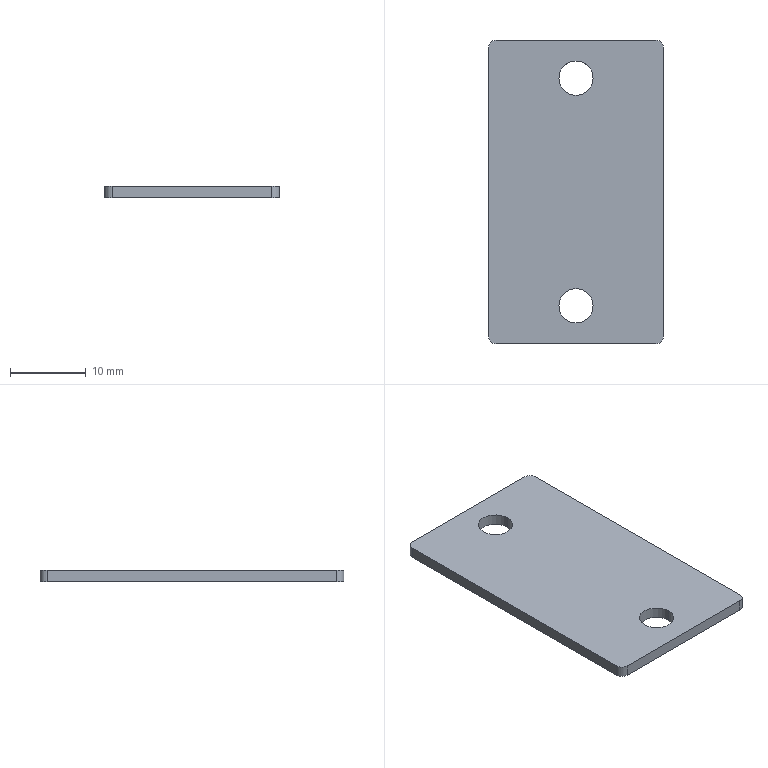Part | STEP file | LE-MX-A-P2_PN_0009 | 1 solid | 14 faces | box 23 x 40 x 1.5 mm | volume 1331 mm3 | cylinder 8 | plane 6 | commonest cylinder face diameters 2 x4 4.5 x4
STEP:
#1=CARTESIAN_POINT('',(2.25,15.,1.5));
#2=VERTEX_POINT('',#1);
#3=CARTESIAN_POINT('',(-2.25,15.,1.5));
#4=VERTEX_POINT('',#3);
#5=CARTESIAN_POINT('',(0.,15.,1.5));
#6=DIRECTION('',(0.,0.,-1.));
#7=DIRECTION('',(-1.,0.,0.));
#8=AXIS2_PLACEMENT_3D('',#5,#6,#7);
#9=CIRCLE('',#8,2.25);
#10=EDGE_CURVE('',#2,#4,#9,.T.);
#11=ORIENTED_EDGE('',*,*,#10,.F.);
#12=CARTESIAN_POINT('',(2.25,15.,0.));
#13=VERTEX_POINT('',#12);
#14=CARTESIAN_POINT('',(2.25,15.,1.5));
#15=DIRECTION('',(0.,0.,-1.));
#16=VECTOR('',#15,1000.);
#17=LINE('',#14,#16);
#18=EDGE_CURVE('',#2,#13,#17,.T.);
#19=ORIENTED_EDGE('',*,*,#18,.T.);
#20=CARTESIAN_POINT('',(-2.25,15.,0.));
#21=VERTEX_POINT('',#20);
#22=CARTESIAN_POINT('',(0.,15.,0.));
#23=DIRECTION('',(0.,0.,1.));
#24=DIRECTION('',(-1.,0.,0.));
#25=AXIS2_PLACEMENT_3D('',#22,#23,#24);
#26=CIRCLE('',#25,2.25);
#27=EDGE_CURVE('',#21,#13,#26,.T.);
#28=ORIENTED_EDGE('',*,*,#27,.F.);
#29=CARTESIAN_POINT('',(-2.25,15.,1.5));
#30=DIRECTION('',(0.,0.,-1.));
#31=VECTOR('',#30,1000.);
#32=LINE('',#29,#31);
#33=EDGE_CURVE('',#4,#21,#32,.T.);
#34=ORIENTED_EDGE('',*,*,#33,.F.);
#35=EDGE_LOOP('',(#11,#19,#28,#34));
#36=FACE_OUTER_BOUND('',#35,.T.);
#37=CARTESIAN_POINT('',(0.,15.,1.5));
#38=DIRECTION('',(0.,0.,-1.));
#39=DIRECTION('',(-1.,0.,0.));
#40=AXIS2_PLACEMENT_3D('',#37,#38,#39);
#41=CYLINDRICAL_SURFACE('',#40,2.25);
#42=ADVANCED_FACE('',(#36),#41,.F.);
#43=CARTESIAN_POINT('',(2.25,-15.,1.5));
#44=VERTEX_POINT('',#43);
#45=CARTESIAN_POINT('',(-2.25,-15.,1.5));
#46=VERTEX_POINT('',#45);
#47=CARTESIAN_POINT('',(0.,-15.,1.5));
#48=DIRECTION('',(0.,0.,-1.));
#49=DIRECTION('',(-1.,0.,0.));
#50=AXIS2_PLACEMENT_3D('',#47,#48,#49);
#51=CIRCLE('',#50,2.25);
#52=EDGE_CURVE('',#44,#46,#51,.T.);
#53=ORIENTED_EDGE('',*,*,#52,.F.);
#54=CARTESIAN_POINT('',(2.25,-15.,0.));
#55=VERTEX_POINT('',#54);
#56=CARTESIAN_POINT('',(2.25,-15.,1.5));
#57=DIRECTION('',(0.,0.,-1.));
#58=VECTOR('',#57,1000.);
#59=LINE('',#56,#58);
#60=EDGE_CURVE('',#44,#55,#59,.T.);
#61=ORIENTED_EDGE('',*,*,#60,.T.);
#62=CARTESIAN_POINT('',(-2.25,-15.,0.));
#63=VERTEX_POINT('',#62);
#64=CARTESIAN_POINT('',(0.,-15.,0.));
#65=DIRECTION('',(0.,0.,1.));
#66=DIRECTION('',(-1.,0.,0.));
#67=AXIS2_PLACEMENT_3D('',#64,#65,#66);
#68=CIRCLE('',#67,2.25);
#69=EDGE_CURVE('',#63,#55,#68,.T.);
#70=ORIENTED_EDGE('',*,*,#69,.F.);
#71=CARTESIAN_POINT('',(-2.25,-15.,1.5));
#72=DIRECTION('',(0.,0.,-1.));
#73=VECTOR('',#72,1000.);
#74=LINE('',#71,#73);
#75=EDGE_CURVE('',#46,#63,#74,.T.);
#76=ORIENTED_EDGE('',*,*,#75,.F.);
#77=EDGE_LOOP('',(#53,#61,#70,#76));
#78=FACE_OUTER_BOUND('',#77,.T.);
#79=CARTESIAN_POINT('',(0.,-15.,1.5));
#80=DIRECTION('',(0.,0.,-1.));
#81=DIRECTION('',(-1.,0.,0.));
#82=AXIS2_PLACEMENT_3D('',#79,#80,#81);
#83=CYLINDRICAL_SURFACE('',#82,2.25);
#84=ADVANCED_FACE('',(#78),#83,.F.);
#85=CARTESIAN_POINT('',(0.,15.,1.5));
#86=DIRECTION('',(0.,0.,-1.));
#87=DIRECTION('',(-1.,0.,0.));
#88=AXIS2_PLACEMENT_3D('',#85,#86,#87);
#89=CIRCLE('',#88,2.25);
#90=EDGE_CURVE('',#4,#2,#89,.T.);
#91=ORIENTED_EDGE('',*,*,#90,.T.);
#92=ORIENTED_EDGE('',*,*,#10,.T.);
#93=EDGE_LOOP('',(#91,#92));
#94=FACE_BOUND('',#93,.T.);
#95=CARTESIAN_POINT('',(-10.5,20.,1.5));
#96=VERTEX_POINT('',#95);
#97=CARTESIAN_POINT('',(-11.5,19.,1.5));
#98=VERTEX_POINT('',#97);
#99=CARTESIAN_POINT('',(-10.5,19.,1.5));
#100=DIRECTION('',(0.,0.,1.));
#101=DIRECTION('',(-1.,0.,0.));
#102=AXIS2_PLACEMENT_3D('',#99,#100,#101);
#103=CIRCLE('',#102,1.);
#104=EDGE_CURVE('',#96,#98,#103,.T.);
#105=ORIENTED_EDGE('',*,*,#104,.T.);
#106=CARTESIAN_POINT('',(-11.5,-19.,1.5));
#107=VERTEX_POINT('',#106);
#108=CARTESIAN_POINT('',(-11.5,-19.,1.5));
#109=DIRECTION('',(0.,-1.,0.));
#110=VECTOR('',#109,1000.);
#111=LINE('',#108,#110);
#112=EDGE_CURVE('',#98,#107,#111,.T.);
#113=ORIENTED_EDGE('',*,*,#112,.T.);
#114=CARTESIAN_POINT('',(-10.5,-20.,1.5));
#115=VERTEX_POINT('',#114);
#116=CARTESIAN_POINT('',(-10.5,-19.,1.5));
#117=DIRECTION('',(0.,0.,1.));
#118=DIRECTION('',(-1.,0.,0.));
#119=AXIS2_PLACEMENT_3D('',#116,#117,#118);
#120=CIRCLE('',#119,1.);
#121=EDGE_CURVE('',#107,#115,#120,.T.);
#122=ORIENTED_EDGE('',*,*,#121,.T.);
#123=CARTESIAN_POINT('',(10.5,-20.,1.5));
#124=VERTEX_POINT('',#123);
#125=CARTESIAN_POINT('',(-10.5,-20.,1.5));
#126=DIRECTION('',(1.,0.,0.));
#127=VECTOR('',#126,1000.);
#128=LINE('',#125,#127);
#129=EDGE_CURVE('',#115,#124,#128,.T.);
#130=ORIENTED_EDGE('',*,*,#129,.T.);
#131=CARTESIAN_POINT('',(11.5,-19.,1.5));
#132=VERTEX_POINT('',#131);
#133=CARTESIAN_POINT('',(10.5,-19.,1.5));
#134=DIRECTION('',(0.,0.,1.));
#135=DIRECTION('',(-1.,0.,0.));
#136=AXIS2_PLACEMENT_3D('',#133,#134,#135);
#137=CIRCLE('',#136,1.);
#138=EDGE_CURVE('',#124,#132,#137,.T.);
#139=ORIENTED_EDGE('',*,*,#138,.T.);
#140=CARTESIAN_POINT('',(11.5,19.,1.5));
#141=VERTEX_POINT('',#140);
#142=CARTESIAN_POINT('',(11.5,-19.,1.5));
#143=DIRECTION('',(0.,1.,0.));
#144=VECTOR('',#143,1000.);
#145=LINE('',#142,#144);
#146=EDGE_CURVE('',#132,#141,#145,.T.);
#147=ORIENTED_EDGE('',*,*,#146,.T.);
#148=CARTESIAN_POINT('',(10.5,20.,1.5));
#149=VERTEX_POINT('',#148);
#150=CARTESIAN_POINT('',(10.5,19.,1.5));
#151=DIRECTION('',(0.,0.,1.));
#152=DIRECTION('',(-1.,0.,0.));
#153=AXIS2_PLACEMENT_3D('',#150,#151,#152);
#154=CIRCLE('',#153,1.);
#155=EDGE_CURVE('',#141,#149,#154,.T.);
#156=ORIENTED_EDGE('',*,*,#155,.T.);
#157=CARTESIAN_POINT('',(-10.5,20.,1.5));
#158=DIRECTION('',(-1.,0.,0.));
#159=VECTOR('',#158,1000.);
#160=LINE('',#157,#159);
#161=EDGE_CURVE('',#149,#96,#160,.T.);
#162=ORIENTED_EDGE('',*,*,#161,.T.);
#163=EDGE_LOOP('',(#105,#113,#122,#130,#139,#147,#156,#162));
#164=FACE_OUTER_BOUND('',#163,.T.);
#165=CARTESIAN_POINT('',(0.,-15.,1.5));
#166=DIRECTION('',(0.,0.,-1.));
#167=DIRECTION('',(-1.,0.,0.));
#168=AXIS2_PLACEMENT_3D('',#165,#166,#167);
#169=CIRCLE('',#168,2.25);
#170=EDGE_CURVE('',#46,#44,#169,.T.);
#171=ORIENTED_EDGE('',*,*,#170,.T.);
#172=ORIENTED_EDGE('',*,*,#52,.T.);
#173=EDGE_LOOP('',(#171,#172));
#174=FACE_BOUND('',#173,.T.);
#175=CARTESIAN_POINT('',(-10.5,-19.,1.5));
#176=DIRECTION('',(0.,0.,1.));
#177=DIRECTION('',(1.,0.,0.));
#178=AXIS2_PLACEMENT_3D('',#175,#176,#177);
#179=PLANE('',#178);
#180=ADVANCED_FACE('',(#94,#164,#174),#179,.T.);
#181=ORIENTED_EDGE('',*,*,#18,.F.);
#182=ORIENTED_EDGE('',*,*,#90,.F.);
#183=ORIENTED_EDGE('',*,*,#33,.T.);
#184=CARTESIAN_POINT('',(0.,15.,0.));
#185=DIRECTION('',(0.,0.,1.));
#186=DIRECTION('',(-1.,0.,0.));
#187=AXIS2_PLACEMENT_3D('',#184,#185,#186);
#188=CIRCLE('',#187,2.25);
#189=EDGE_CURVE('',#13,#21,#188,.T.);
#190=ORIENTED_EDGE('',*,*,#189,.F.);
#191=EDGE_LOOP('',(#181,#182,#183,#190));
#192=FACE_OUTER_BOUND('',#191,.T.);
#193=CARTESIAN_POINT('',(0.,15.,1.5));
#194=DIRECTION('',(0.,0.,-1.));
#195=DIRECTION('',(-1.,0.,0.));
#196=AXIS2_PLACEMENT_3D('',#193,#194,#195);
#197=CYLINDRICAL_SURFACE('',#196,2.25);
#198=ADVANCED_FACE('',(#192),#197,.F.);
#199=CARTESIAN_POINT('',(-11.5,-19.,0.));
#200=VERTEX_POINT('',#199);
#201=CARTESIAN_POINT('',(-11.5,-19.,1.5));
#202=DIRECTION('',(0.,0.,-1.));
#203=VECTOR('',#202,1000.);
#204=LINE('',#201,#203);
#205=EDGE_CURVE('',#107,#200,#204,.T.);
#206=ORIENTED_EDGE('',*,*,#205,.F.);
#207=ORIENTED_EDGE('',*,*,#112,.F.);
#208=CARTESIAN_POINT('',(-11.5,19.,0.));
#209=VERTEX_POINT('',#208);
#210=CARTESIAN_POINT('',(-11.5,19.,1.5));
#211=DIRECTION('',(0.,0.,1.));
#212=VECTOR('',#211,1000.);
#213=LINE('',#210,#212);
#214=EDGE_CURVE('',#209,#98,#213,.T.);
#215=ORIENTED_EDGE('',*,*,#214,.F.);
#216=CARTESIAN_POINT('',(-11.5,19.,0.));
#217=DIRECTION('',(0.,1.,0.));
#218=VECTOR('',#217,1000.);
#219=LINE('',#216,#218);
#220=EDGE_CURVE('',#200,#209,#219,.T.);
#221=ORIENTED_EDGE('',*,*,#220,.F.);
#222=EDGE_LOOP('',(#206,#207,#215,#221));
#223=FACE_OUTER_BOUND('',#222,.T.);
#224=CARTESIAN_POINT('',(-11.5,19.,1.5));
#225=DIRECTION('',(1.,0.,0.));
#226=DIRECTION('',(0.,0.,-1.));
#227=AXIS2_PLACEMENT_3D('',#224,#225,#226);
#228=PLANE('',#227);
#229=ADVANCED_FACE('',(#223),#228,.F.);
#230=ORIENTED_EDGE('',*,*,#104,.F.);
#231=CARTESIAN_POINT('',(-10.5,20.,0.));
#232=VERTEX_POINT('',#231);
#233=CARTESIAN_POINT('',(-10.5,20.,1.5));
#234=DIRECTION('',(0.,0.,-1.));
#235=VECTOR('',#234,1000.);
#236=LINE('',#233,#235);
#237=EDGE_CURVE('',#96,#232,#236,.T.);
#238=ORIENTED_EDGE('',*,*,#237,.T.);
#239=CARTESIAN_POINT('',(-10.5,19.,0.));
#240=DIRECTION('',(0.,0.,1.));
#241=DIRECTION('',(-1.,0.,0.));
#242=AXIS2_PLACEMENT_3D('',#239,#240,#241);
#243=CIRCLE('',#242,1.);
#244=EDGE_CURVE('',#232,#209,#243,.T.);
#245=ORIENTED_EDGE('',*,*,#244,.T.);
#246=ORIENTED_EDGE('',*,*,#214,.T.);
#247=EDGE_LOOP('',(#230,#238,#245,#246));
#248=FACE_OUTER_BOUND('',#247,.T.);
#249=CARTESIAN_POINT('',(-10.5,19.,1.5));
#250=DIRECTION('',(0.,0.,-1.));
#251=DIRECTION('',(-1.,0.,0.));
#252=AXIS2_PLACEMENT_3D('',#249,#250,#251);
#253=CYLINDRICAL_SURFACE('',#252,1.);
#254=ADVANCED_FACE('',(#248),#253,.T.);
#255=ORIENTED_EDGE('',*,*,#237,.F.);
#256=ORIENTED_EDGE('',*,*,#161,.F.);
#257=CARTESIAN_POINT('',(10.5,20.,0.));
#258=VERTEX_POINT('',#257);
#259=CARTESIAN_POINT('',(10.5,20.,1.5));
#260=DIRECTION('',(0.,0.,1.));
#261=VECTOR('',#260,1000.);
#262=LINE('',#259,#261);
#263=EDGE_CURVE('',#258,#149,#262,.T.);
#264=ORIENTED_EDGE('',*,*,#263,.F.);
#265=CARTESIAN_POINT('',(10.5,20.,0.));
#266=DIRECTION('',(1.,0.,0.));
#267=VECTOR('',#266,1000.);
#268=LINE('',#265,#267);
#269=EDGE_CURVE('',#232,#258,#268,.T.);
#270=ORIENTED_EDGE('',*,*,#269,.F.);
#271=EDGE_LOOP('',(#255,#256,#264,#270));
#272=FACE_OUTER_BOUND('',#271,.T.);
#273=CARTESIAN_POINT('',(10.5,20.,1.5));
#274=DIRECTION('',(0.,-1.,0.));
#275=DIRECTION('',(0.,0.,-1.));
#276=AXIS2_PLACEMENT_3D('',#273,#274,#275);
#277=PLANE('',#276);
#278=ADVANCED_FACE('',(#272),#277,.F.);
#279=ORIENTED_EDGE('',*,*,#155,.F.);
#280=CARTESIAN_POINT('',(11.5,19.,0.));
#281=VERTEX_POINT('',#280);
#282=CARTESIAN_POINT('',(11.5,19.,1.5));
#283=DIRECTION('',(0.,0.,-1.));
#284=VECTOR('',#283,1000.);
#285=LINE('',#282,#284);
#286=EDGE_CURVE('',#141,#281,#285,.T.);
#287=ORIENTED_EDGE('',*,*,#286,.T.);
#288=CARTESIAN_POINT('',(10.5,19.,0.));
#289=DIRECTION('',(0.,0.,1.));
#290=DIRECTION('',(-1.,0.,0.));
#291=AXIS2_PLACEMENT_3D('',#288,#289,#290);
#292=CIRCLE('',#291,1.);
#293=EDGE_CURVE('',#281,#258,#292,.T.);
#294=ORIENTED_EDGE('',*,*,#293,.T.);
#295=ORIENTED_EDGE('',*,*,#263,.T.);
#296=EDGE_LOOP('',(#279,#287,#294,#295));
#297=FACE_OUTER_BOUND('',#296,.T.);
#298=CARTESIAN_POINT('',(10.5,19.,1.5));
#299=DIRECTION('',(0.,0.,-1.));
#300=DIRECTION('',(-1.,0.,0.));
#301=AXIS2_PLACEMENT_3D('',#298,#299,#300);
#302=CYLINDRICAL_SURFACE('',#301,1.);
#303=ADVANCED_FACE('',(#297),#302,.T.);
#304=ORIENTED_EDGE('',*,*,#286,.F.);
#305=ORIENTED_EDGE('',*,*,#146,.F.);
#306=CARTESIAN_POINT('',(11.5,-19.,0.));
#307=VERTEX_POINT('',#306);
#308=CARTESIAN_POINT('',(11.5,-19.,1.5));
#309=DIRECTION('',(0.,0.,1.));
#310=VECTOR('',#309,1000.);
#311=LINE('',#308,#310);
#312=EDGE_CURVE('',#307,#132,#311,.T.);
#313=ORIENTED_EDGE('',*,*,#312,.F.);
#314=CARTESIAN_POINT('',(11.5,-19.,0.));
#315=DIRECTION('',(0.,-1.,0.));
#316=VECTOR('',#315,1000.);
#317=LINE('',#314,#316);
#318=EDGE_CURVE('',#281,#307,#317,.T.);
#319=ORIENTED_EDGE('',*,*,#318,.F.);
#320=EDGE_LOOP('',(#304,#305,#313,#319));
#321=FACE_OUTER_BOUND('',#320,.T.);
#322=CARTESIAN_POINT('',(11.5,-19.,1.5));
#323=DIRECTION('',(-1.,0.,0.));
#324=DIRECTION('',(0.,0.,1.));
#325=AXIS2_PLACEMENT_3D('',#322,#323,#324);
#326=PLANE('',#325);
#327=ADVANCED_FACE('',(#321),#326,.F.);
#328=ORIENTED_EDGE('',*,*,#138,.F.);
#329=CARTESIAN_POINT('',(10.5,-20.,0.));
#330=VERTEX_POINT('',#329);
#331=CARTESIAN_POINT('',(10.5,-20.,1.5));
#332=DIRECTION('',(0.,0.,-1.));
#333=VECTOR('',#332,1000.);
#334=LINE('',#331,#333);
#335=EDGE_CURVE('',#124,#330,#334,.T.);
#336=ORIENTED_EDGE('',*,*,#335,.T.);
#337=CARTESIAN_POINT('',(10.5,-19.,0.));
#338=DIRECTION('',(0.,0.,1.));
#339=DIRECTION('',(-1.,0.,0.));
#340=AXIS2_PLACEMENT_3D('',#337,#338,#339);
#341=CIRCLE('',#340,1.);
#342=EDGE_CURVE('',#330,#307,#341,.T.);
#343=ORIENTED_EDGE('',*,*,#342,.T.);
#344=ORIENTED_EDGE('',*,*,#312,.T.);
#345=EDGE_LOOP('',(#328,#336,#343,#344));
#346=FACE_OUTER_BOUND('',#345,.T.);
#347=CARTESIAN_POINT('',(10.5,-19.,1.5));
#348=DIRECTION('',(0.,0.,-1.));
#349=DIRECTION('',(-1.,0.,0.));
#350=AXIS2_PLACEMENT_3D('',#347,#348,#349);
#351=CYLINDRICAL_SURFACE('',#350,1.);
#352=ADVANCED_FACE('',(#346),#351,.T.);
#353=ORIENTED_EDGE('',*,*,#335,.F.);
#354=ORIENTED_EDGE('',*,*,#129,.F.);
#355=CARTESIAN_POINT('',(-10.5,-20.,0.));
#356=VERTEX_POINT('',#355);
#357=CARTESIAN_POINT('',(-10.5,-20.,1.5));
#358=DIRECTION('',(0.,0.,1.));
#359=VECTOR('',#358,1000.);
#360=LINE('',#357,#359);
#361=EDGE_CURVE('',#356,#115,#360,.T.);
#362=ORIENTED_EDGE('',*,*,#361,.F.);
#363=CARTESIAN_POINT('',(-10.5,-20.,0.));
#364=DIRECTION('',(-1.,0.,0.));
#365=VECTOR('',#364,1000.);
#366=LINE('',#363,#365);
#367=EDGE_CURVE('',#330,#356,#366,.T.);
#368=ORIENTED_EDGE('',*,*,#367,.F.);
#369=EDGE_LOOP('',(#353,#354,#362,#368));
#370=FACE_OUTER_BOUND('',#369,.T.);
#371=CARTESIAN_POINT('',(-10.5,-20.,1.5));
#372=DIRECTION('',(0.,1.,0.));
#373=DIRECTION('',(0.,0.,1.));
#374=AXIS2_PLACEMENT_3D('',#371,#372,#373);
#375=PLANE('',#374);
#376=ADVANCED_FACE('',(#370),#375,.F.);
#377=ORIENTED_EDGE('',*,*,#121,.F.);
#378=ORIENTED_EDGE('',*,*,#205,.T.);
#379=CARTESIAN_POINT('',(-10.5,-19.,0.));
#380=DIRECTION('',(0.,0.,1.));
#381=DIRECTION('',(-1.,0.,0.));
#382=AXIS2_PLACEMENT_3D('',#379,#380,#381);
#383=CIRCLE('',#382,1.);
#384=EDGE_CURVE('',#200,#356,#383,.T.);
#385=ORIENTED_EDGE('',*,*,#384,.T.);
#386=ORIENTED_EDGE('',*,*,#361,.T.);
#387=EDGE_LOOP('',(#377,#378,#385,#386));
#388=FACE_OUTER_BOUND('',#387,.T.);
#389=CARTESIAN_POINT('',(-10.5,-19.,1.5));
#390=DIRECTION('',(0.,0.,-1.));
#391=DIRECTION('',(-1.,0.,0.));
#392=AXIS2_PLACEMENT_3D('',#389,#390,#391);
#393=CYLINDRICAL_SURFACE('',#392,1.);
#394=ADVANCED_FACE('',(#388),#393,.T.);
#395=ORIENTED_EDGE('',*,*,#60,.F.);
#396=ORIENTED_EDGE('',*,*,#170,.F.);
#397=ORIENTED_EDGE('',*,*,#75,.T.);
#398=CARTESIAN_POINT('',(0.,-15.,0.));
#399=DIRECTION('',(0.,0.,1.));
#400=DIRECTION('',(-1.,0.,0.));
#401=AXIS2_PLACEMENT_3D('',#398,#399,#400);
#402=CIRCLE('',#401,2.25);
#403=EDGE_CURVE('',#55,#63,#402,.T.);
#404=ORIENTED_EDGE('',*,*,#403,.F.);
#405=EDGE_LOOP('',(#395,#396,#397,#404));
#406=FACE_OUTER_BOUND('',#405,.T.);
#407=CARTESIAN_POINT('',(0.,-15.,1.5));
#408=DIRECTION('',(0.,0.,-1.));
#409=DIRECTION('',(-1.,0.,0.));
#410=AXIS2_PLACEMENT_3D('',#407,#408,#409);
#411=CYLINDRICAL_SURFACE('',#410,2.25);
#412=ADVANCED_FACE('',(#406),#411,.F.);
#413=ORIENTED_EDGE('',*,*,#27,.T.);
#414=ORIENTED_EDGE('',*,*,#189,.T.);
#415=EDGE_LOOP('',(#413,#414));
#416=FACE_BOUND('',#415,.T.);
#417=ORIENTED_EDGE('',*,*,#220,.T.);
#418=ORIENTED_EDGE('',*,*,#244,.F.);
#419=ORIENTED_EDGE('',*,*,#269,.T.);
#420=ORIENTED_EDGE('',*,*,#293,.F.);
#421=ORIENTED_EDGE('',*,*,#318,.T.);
#422=ORIENTED_EDGE('',*,*,#342,.F.);
#423=ORIENTED_EDGE('',*,*,#367,.T.);
#424=ORIENTED_EDGE('',*,*,#384,.F.);
#425=EDGE_LOOP('',(#417,#418,#419,#420,#421,#422,#423,#424));
#426=FACE_OUTER_BOUND('',#425,.T.);
#427=ORIENTED_EDGE('',*,*,#69,.T.);
#428=ORIENTED_EDGE('',*,*,#403,.T.);
#429=EDGE_LOOP('',(#427,#428));
#430=FACE_BOUND('',#429,.T.);
#431=CARTESIAN_POINT('',(-10.5,-19.,0.));
#432=DIRECTION('',(0.,0.,1.));
#433=DIRECTION('',(1.,0.,0.));
#434=AXIS2_PLACEMENT_3D('',#431,#432,#433);
#435=PLANE('',#434);
#436=ADVANCED_FACE('',(#416,#426,#430),#435,.F.);
#437=CLOSED_SHELL('',(#42,#84,#180,#198,#229,#254,#278,#303,#327,#352,#376,#394,#412,#436));
#438=MANIFOLD_SOLID_BREP('',#437);
#439=CARTESIAN_POINT('',(0.,0.,0.));
#440=DIRECTION('',(0.,0.,1.));
#441=DIRECTION('',(1.,0.,0.));
#442=AXIS2_PLACEMENT_3D('',#439,#440,#441);
#443=(LENGTH_UNIT()NAMED_UNIT(*)SI_UNIT(.MILLI.,.METRE.));
#444=UNCERTAINTY_MEASURE_WITH_UNIT(LENGTH_MEASURE(0.00001),#443,'','');
#445=(NAMED_UNIT(*)PLANE_ANGLE_UNIT()SI_UNIT($,.RADIAN.));
#446=(NAMED_UNIT(*)SI_UNIT($,.STERADIAN.)SOLID_ANGLE_UNIT());
#447=(GEOMETRIC_REPRESENTATION_CONTEXT(3)GLOBAL_UNCERTAINTY_ASSIGNED_CONTEXT((#444))GLOBAL_UNIT_ASSIGNED_CONTEXT((#443,#445,#446))REPRESENTATION_CONTEXT('',''));
#448=ADVANCED_BREP_SHAPE_REPRESENTATION('',(#438,#442),#447);